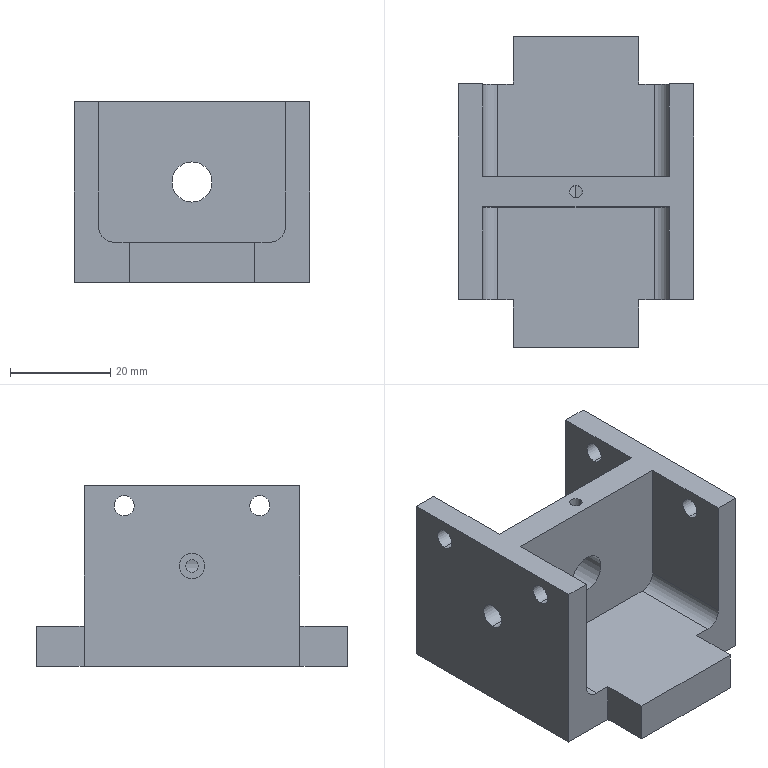Part | SolidWorks | features ICE 6, 3DProfileFeature 2, HoleWzd 2, Extrusion 1, Fillet 1 | 1 solid | 43 faces | box 47 x 62 x 36 mm | volume 37251 mm3 | plane 23 | cylinder 20 | commonest cylinder face diameters 4 x8 2.5 x4 6 x4 5 x2 8 x2
STEP:
#1=CARTESIAN_POINT('',(-9.5,0.,17.5));
#2=VERTEX_POINT('',#1);
#3=CARTESIAN_POINT('',(-9.5,0.,22.5));
#4=VERTEX_POINT('',#3);
#5=CARTESIAN_POINT('',(-9.5,0.,20.));
#6=DIRECTION('',(-1.,0.,0.));
#7=DIRECTION('',(0.,0.,1.));
#8=AXIS2_PLACEMENT_3D('',#5,#6,#7);
#9=CIRCLE('',#8,2.5);
#10=EDGE_CURVE('',#2,#4,#9,.T.);
#11=ORIENTED_EDGE('',*,*,#10,.F.);
#12=CARTESIAN_POINT('',(-23.5,0.,17.5));
#13=VERTEX_POINT('',#12);
#14=CARTESIAN_POINT('',(-9.5,0.,17.5));
#15=DIRECTION('',(-1.,0.,0.));
#16=VECTOR('',#15,1000.);
#17=LINE('',#14,#16);
#18=EDGE_CURVE('',#2,#13,#17,.T.);
#19=ORIENTED_EDGE('',*,*,#18,.T.);
#20=CARTESIAN_POINT('',(-23.5,0.,22.5));
#21=VERTEX_POINT('',#20);
#22=CARTESIAN_POINT('',(-23.5,0.,20.));
#23=DIRECTION('',(-1.,0.,0.));
#24=DIRECTION('',(0.,0.,1.));
#25=AXIS2_PLACEMENT_3D('',#22,#23,#24);
#26=CIRCLE('',#25,2.5);
#27=EDGE_CURVE('',#13,#21,#26,.T.);
#28=ORIENTED_EDGE('',*,*,#27,.T.);
#29=CARTESIAN_POINT('',(-9.5,0.,22.5));
#30=DIRECTION('',(-1.,0.,0.));
#31=VECTOR('',#30,1000.);
#32=LINE('',#29,#31);
#33=EDGE_CURVE('',#4,#21,#32,.T.);
#34=ORIENTED_EDGE('',*,*,#33,.F.);
#35=EDGE_LOOP('',(#11,#19,#28,#34));
#36=FACE_OUTER_BOUND('',#35,.T.);
#37=CARTESIAN_POINT('',(-9.5,0.,20.));
#38=DIRECTION('',(-1.,0.,0.));
#39=DIRECTION('',(0.,0.,1.));
#40=AXIS2_PLACEMENT_3D('',#37,#38,#39);
#41=CYLINDRICAL_SURFACE('',#40,2.5);
#42=ADVANCED_FACE('',(#36),#41,.F.);
#43=CARTESIAN_POINT('',(-1.25,0.,23.8));
#44=VERTEX_POINT('',#43);
#45=CARTESIAN_POINT('',(0.,-1.25,24.));
#46=VERTEX_POINT('',#45);
#47=CARTESIAN_POINT('',(-1.25,0.,23.8));
#48=CARTESIAN_POINT('',(-1.25,-0.1648,23.8));
#49=CARTESIAN_POINT('',(-1.217,-0.3295,23.811));
#50=CARTESIAN_POINT('',(-1.092,-0.6305,23.849));
#51=CARTESIAN_POINT('',(-0.9987,-0.769,23.875));
#52=CARTESIAN_POINT('',(-0.7696,-0.9982,23.927));
#53=CARTESIAN_POINT('',(-0.6317,-1.091,23.953));
#54=CARTESIAN_POINT('',(-0.3299,-1.217,23.989));
#55=CARTESIAN_POINT('',(-0.1663,-1.25,24.));
#56=CARTESIAN_POINT('',(0.,-1.25,24.));
#57=B_SPLINE_CURVE_WITH_KNOTS('',3,(#47,#48,#49,#50,#51,#52,#53,#54,#55,#56),.UNSPECIFIED.,.F.,.F.,(4,2,2,2,4),(0.005899,0.00639,0.006882,0.007373,0.007865),.UNSPECIFIED.);
#58=EDGE_CURVE('',#44,#46,#57,.T.);
#59=ORIENTED_EDGE('',*,*,#58,.F.);
#60=CARTESIAN_POINT('',(-1.25,0.,36.));
#61=VERTEX_POINT('',#60);
#62=CARTESIAN_POINT('',(-1.25,0.,36.));
#63=DIRECTION('',(0.,0.,1.));
#64=VECTOR('',#63,1000.);
#65=LINE('',#62,#64);
#66=EDGE_CURVE('',#44,#61,#65,.T.);
#67=ORIENTED_EDGE('',*,*,#66,.T.);
#68=CARTESIAN_POINT('',(1.25,0.,36.));
#69=VERTEX_POINT('',#68);
#70=CARTESIAN_POINT('',(0.,0.,36.));
#71=DIRECTION('',(0.,0.,1.));
#72=DIRECTION('',(1.,0.,0.));
#73=AXIS2_PLACEMENT_3D('',#70,#71,#72);
#74=CIRCLE('',#73,1.25);
#75=EDGE_CURVE('',#61,#69,#74,.T.);
#76=ORIENTED_EDGE('',*,*,#75,.T.);
#77=CARTESIAN_POINT('',(1.25,0.,23.8));
#78=VERTEX_POINT('',#77);
#79=CARTESIAN_POINT('',(1.25,0.,36.));
#80=DIRECTION('',(0.,0.,1.));
#81=VECTOR('',#80,1000.);
#82=LINE('',#79,#81);
#83=EDGE_CURVE('',#78,#69,#82,.T.);
#84=ORIENTED_EDGE('',*,*,#83,.F.);
#85=CARTESIAN_POINT('',(0.,-1.25,24.));
#86=CARTESIAN_POINT('',(0.1664,-1.25,24.));
#87=CARTESIAN_POINT('',(0.3295,-1.217,23.989));
#88=CARTESIAN_POINT('',(0.6319,-1.091,23.953));
#89=CARTESIAN_POINT('',(0.7699,-0.998,23.927));
#90=CARTESIAN_POINT('',(0.9989,-0.7687,23.875));
#91=CARTESIAN_POINT('',(1.092,-0.63,23.849));
#92=CARTESIAN_POINT('',(1.217,-0.3295,23.811));
#93=CARTESIAN_POINT('',(1.25,-0.1643,23.8));
#94=CARTESIAN_POINT('',(1.25,0.,23.8));
#95=B_SPLINE_CURVE_WITH_KNOTS('',3,(#85,#86,#87,#88,#89,#90,#91,#92,#93,#94),.UNSPECIFIED.,.F.,.F.,(4,2,2,2,4),(0.,0.0004918,0.0009835,0.001475,0.001967),.UNSPECIFIED.);
#96=EDGE_CURVE('',#46,#78,#95,.T.);
#97=ORIENTED_EDGE('',*,*,#96,.F.);
#98=EDGE_LOOP('',(#59,#67,#76,#84,#97));
#99=FACE_OUTER_BOUND('',#98,.T.);
#100=CARTESIAN_POINT('',(0.,0.,36.));
#101=DIRECTION('',(0.,0.,1.));
#102=DIRECTION('',(1.,0.,0.));
#103=AXIS2_PLACEMENT_3D('',#100,#101,#102);
#104=CYLINDRICAL_SURFACE('',#103,1.25);
#105=ADVANCED_FACE('',(#99),#104,.F.);
#106=CARTESIAN_POINT('',(-3.8,0.,21.25));
#107=VERTEX_POINT('',#106);
#108=CARTESIAN_POINT('',(-3.8,0.,18.75));
#109=VERTEX_POINT('',#108);
#110=CARTESIAN_POINT('',(-3.8,0.,21.25));
#111=CARTESIAN_POINT('',(-3.8,0.1663,21.25));
#112=CARTESIAN_POINT('',(-3.811,0.3294,21.217));
#113=CARTESIAN_POINT('',(-3.849,0.6316,21.091));
#114=CARTESIAN_POINT('',(-3.875,0.7696,20.998));
#115=CARTESIAN_POINT('',(-3.927,0.9986,20.769));
#116=CARTESIAN_POINT('',(-3.953,1.092,20.631));
#117=CARTESIAN_POINT('',(-3.989,1.217,20.33));
#118=CARTESIAN_POINT('',(-4.,1.25,20.165));
#119=CARTESIAN_POINT('',(-4.,1.25,19.918));
#120=CARTESIAN_POINT('',(-3.997,1.242,19.835));
#121=CARTESIAN_POINT('',(-3.988,1.21,19.674));
#122=CARTESIAN_POINT('',(-3.98,1.186,19.596));
#123=CARTESIAN_POINT('',(-3.953,1.091,19.368));
#124=CARTESIAN_POINT('',(-3.927,0.9987,19.231));
#125=CARTESIAN_POINT('',(-3.888,0.8257,19.058));
#126=CARTESIAN_POINT('',(-3.875,0.7631,19.007));
#127=CARTESIAN_POINT('',(-3.851,0.6281,18.916));
#128=CARTESIAN_POINT('',(-3.839,0.555,18.877));
#129=CARTESIAN_POINT('',(-3.811,0.3291,18.783));
#130=CARTESIAN_POINT('',(-3.8,0.1638,18.75));
#131=CARTESIAN_POINT('',(-3.8,0.,18.75));
#132=B_SPLINE_CURVE_WITH_KNOTS('',3,(#110,#111,#112,#113,#114,#115,#116,#117,#118,#119,#120,#121,#122,#123,#124,#125,#126,#127,#128,#129,#130,#131),.UNSPECIFIED.,.F.,.F.,(4,2,2,2,2,2,2,2,2,2,4),(0.,0.0004916,0.0009832,0.001475,0.001966,0.002212,0.002458,0.00295,0.003195,0.003441,0.003933),.UNSPECIFIED.);
#133=EDGE_CURVE('',#107,#109,#132,.T.);
#134=ORIENTED_EDGE('',*,*,#133,.T.);
#135=CARTESIAN_POINT('',(-3.8,0.,18.75));
#136=CARTESIAN_POINT('',(-3.8,-0.1638,18.75));
#137=CARTESIAN_POINT('',(-3.811,-0.3292,18.783));
#138=CARTESIAN_POINT('',(-3.849,-0.6305,18.908));
#139=CARTESIAN_POINT('',(-3.875,-0.7683,19.001));
#140=CARTESIAN_POINT('',(-3.927,-0.9991,19.231));
#141=CARTESIAN_POINT('',(-3.953,-1.091,19.368));
#142=CARTESIAN_POINT('',(-3.98,-1.186,19.596));
#143=CARTESIAN_POINT('',(-3.988,-1.21,19.674));
#144=CARTESIAN_POINT('',(-3.997,-1.242,19.834));
#145=CARTESIAN_POINT('',(-4.,-1.25,19.918));
#146=CARTESIAN_POINT('',(-4.,-1.25,20.165));
#147=CARTESIAN_POINT('',(-3.989,-1.217,20.33));
#148=CARTESIAN_POINT('',(-3.953,-1.091,20.631));
#149=CARTESIAN_POINT('',(-3.927,-0.9985,20.769));
#150=CARTESIAN_POINT('',(-3.875,-0.7694,20.998));
#151=CARTESIAN_POINT('',(-3.849,-0.6315,21.091));
#152=CARTESIAN_POINT('',(-3.811,-0.3299,21.217));
#153=CARTESIAN_POINT('',(-3.8,-0.1663,21.25));
#154=CARTESIAN_POINT('',(-3.8,0.,21.25));
#155=B_SPLINE_CURVE_WITH_KNOTS('',3,(#135,#136,#137,#138,#139,#140,#141,#142,#143,#144,#145,#146,#147,#148,#149,#150,#151,#152,#153,#154),.UNSPECIFIED.,.F.,.F.,(4,2,2,2,2,2,2,2,2,4),(0.003933,0.004424,0.004916,0.005407,0.005653,0.005899,0.00639,0.006882,0.007373,0.007864),.UNSPECIFIED.);
#156=EDGE_CURVE('',#109,#107,#155,.T.);
#157=ORIENTED_EDGE('',*,*,#156,.T.);
#158=EDGE_LOOP('',(#134,#157));
#159=FACE_BOUND('',#158,.T.);
#160=CARTESIAN_POINT('',(0.,-3.,24.));
#161=VERTEX_POINT('',#160);
#162=CARTESIAN_POINT('',(0.,-3.,16.));
#163=VERTEX_POINT('',#162);
#164=CARTESIAN_POINT('',(0.,-3.,20.));
#165=DIRECTION('',(0.,-1.,0.));
#166=DIRECTION('',(0.,0.,1.));
#167=AXIS2_PLACEMENT_3D('',#164,#165,#166);
#168=CIRCLE('',#167,4.);
#169=EDGE_CURVE('',#161,#163,#168,.T.);
#170=ORIENTED_EDGE('',*,*,#169,.T.);
#171=CARTESIAN_POINT('',(0.,3.,16.));
#172=VERTEX_POINT('',#171);
#173=CARTESIAN_POINT('',(0.,-21.501,16.));
#174=DIRECTION('',(0.,1.,0.));
#175=VECTOR('',#174,1000.);
#176=LINE('',#173,#175);
#177=EDGE_CURVE('',#163,#172,#176,.T.);
#178=ORIENTED_EDGE('',*,*,#177,.T.);
#179=CARTESIAN_POINT('',(0.,3.,24.));
#180=VERTEX_POINT('',#179);
#181=CARTESIAN_POINT('',(0.,3.,20.));
#182=DIRECTION('',(0.,1.,0.));
#183=DIRECTION('',(0.,0.,1.));
#184=AXIS2_PLACEMENT_3D('',#181,#182,#183);
#185=CIRCLE('',#184,4.);
#186=EDGE_CURVE('',#172,#180,#185,.T.);
#187=ORIENTED_EDGE('',*,*,#186,.T.);
#188=CARTESIAN_POINT('',(0.,1.25,24.));
#189=VERTEX_POINT('',#188);
#190=CARTESIAN_POINT('',(0.,-21.501,24.));
#191=DIRECTION('',(0.,1.,0.));
#192=VECTOR('',#191,1000.);
#193=LINE('',#190,#192);
#194=EDGE_CURVE('',#189,#180,#193,.T.);
#195=ORIENTED_EDGE('',*,*,#194,.F.);
#196=CARTESIAN_POINT('',(0.,1.25,24.));
#197=CARTESIAN_POINT('',(-0.1638,1.25,24.));
#198=CARTESIAN_POINT('',(-0.3292,1.217,23.989));
#199=CARTESIAN_POINT('',(-0.6307,1.092,23.953));
#200=CARTESIAN_POINT('',(-0.7685,0.9993,23.927));
#201=CARTESIAN_POINT('',(-0.9992,0.7685,23.875));
#202=CARTESIAN_POINT('',(-1.091,0.6322,23.849));
#203=CARTESIAN_POINT('',(-1.186,0.404,23.82));
#204=CARTESIAN_POINT('',(-1.21,0.3258,23.813));
#205=CARTESIAN_POINT('',(-1.242,0.1656,23.802));
#206=CARTESIAN_POINT('',(-1.25,0.08238,23.8));
#207=CARTESIAN_POINT('',(-1.25,0.,23.8));
#208=B_SPLINE_CURVE_WITH_KNOTS('',3,(#196,#197,#198,#199,#200,#201,#202,#203,#204,#205,#206,#207),.UNSPECIFIED.,.F.,.F.,(4,2,2,2,2,4),(0.003933,0.004424,0.004916,0.005407,0.005653,0.005899),.UNSPECIFIED.);
#209=EDGE_CURVE('',#189,#44,#208,.T.);
#210=ORIENTED_EDGE('',*,*,#209,.T.);
#211=ORIENTED_EDGE('',*,*,#58,.T.);
#212=CARTESIAN_POINT('',(0.,-21.501,24.));
#213=DIRECTION('',(0.,1.,0.));
#214=VECTOR('',#213,1000.);
#215=LINE('',#212,#214);
#216=EDGE_CURVE('',#161,#46,#215,.T.);
#217=ORIENTED_EDGE('',*,*,#216,.F.);
#218=EDGE_LOOP('',(#170,#178,#187,#195,#210,#211,#217));
#219=FACE_OUTER_BOUND('',#218,.T.);
#220=CARTESIAN_POINT('',(0.,-21.501,20.));
#221=DIRECTION('',(0.,1.,0.));
#222=DIRECTION('',(0.,0.,1.));
#223=AXIS2_PLACEMENT_3D('',#220,#221,#222);
#224=CYLINDRICAL_SURFACE('',#223,4.);
#225=ADVANCED_FACE('',(#159,#219),#224,.F.);
#226=CARTESIAN_POINT('',(23.5,13.5,34.));
#227=VERTEX_POINT('',#226);
#228=CARTESIAN_POINT('',(23.5,13.5,30.));
#229=VERTEX_POINT('',#228);
#230=CARTESIAN_POINT('',(23.5,13.5,32.));
#231=DIRECTION('',(1.,0.,0.));
#232=DIRECTION('',(0.,0.,1.));
#233=AXIS2_PLACEMENT_3D('',#230,#231,#232);
#234=CIRCLE('',#233,2.);
#235=EDGE_CURVE('',#227,#229,#234,.T.);
#236=ORIENTED_EDGE('',*,*,#235,.T.);
#237=CARTESIAN_POINT('',(18.6,13.5,30.));
#238=VERTEX_POINT('',#237);
#239=CARTESIAN_POINT('',(29.157,13.5,30.));
#240=DIRECTION('',(-1.,0.,0.));
#241=VECTOR('',#240,1000.);
#242=LINE('',#239,#241);
#243=EDGE_CURVE('',#229,#238,#242,.T.);
#244=ORIENTED_EDGE('',*,*,#243,.T.);
#245=CARTESIAN_POINT('',(18.6,13.5,34.));
#246=VERTEX_POINT('',#245);
#247=CARTESIAN_POINT('',(18.6,13.5,32.));
#248=DIRECTION('',(1.,0.,0.));
#249=DIRECTION('',(0.,0.,-1.));
#250=AXIS2_PLACEMENT_3D('',#247,#248,#249);
#251=CIRCLE('',#250,2.);
#252=EDGE_CURVE('',#246,#238,#251,.T.);
#253=ORIENTED_EDGE('',*,*,#252,.F.);
#254=CARTESIAN_POINT('',(29.157,13.5,34.));
#255=DIRECTION('',(-1.,0.,0.));
#256=VECTOR('',#255,1000.);
#257=LINE('',#254,#256);
#258=EDGE_CURVE('',#227,#246,#257,.T.);
#259=ORIENTED_EDGE('',*,*,#258,.F.);
#260=EDGE_LOOP('',(#236,#244,#253,#259));
#261=FACE_OUTER_BOUND('',#260,.T.);
#262=CARTESIAN_POINT('',(29.157,13.5,32.));
#263=DIRECTION('',(-1.,0.,0.));
#264=DIRECTION('',(0.,0.,1.));
#265=AXIS2_PLACEMENT_3D('',#262,#263,#264);
#266=CYLINDRICAL_SURFACE('',#265,2.);
#267=ADVANCED_FACE('',(#261),#266,.F.);
#268=CARTESIAN_POINT('',(23.5,-13.5,34.));
#269=VERTEX_POINT('',#268);
#270=CARTESIAN_POINT('',(23.5,-13.5,30.));
#271=VERTEX_POINT('',#270);
#272=CARTESIAN_POINT('',(23.5,-13.5,32.));
#273=DIRECTION('',(1.,0.,0.));
#274=DIRECTION('',(0.,0.,1.));
#275=AXIS2_PLACEMENT_3D('',#272,#273,#274);
#276=CIRCLE('',#275,2.);
#277=EDGE_CURVE('',#269,#271,#276,.T.);
#278=ORIENTED_EDGE('',*,*,#277,.T.);
#279=CARTESIAN_POINT('',(18.6,-13.5,30.));
#280=VERTEX_POINT('',#279);
#281=CARTESIAN_POINT('',(29.157,-13.5,30.));
#282=DIRECTION('',(-1.,0.,0.));
#283=VECTOR('',#282,1000.);
#284=LINE('',#281,#283);
#285=EDGE_CURVE('',#271,#280,#284,.T.);
#286=ORIENTED_EDGE('',*,*,#285,.T.);
#287=CARTESIAN_POINT('',(18.6,-13.5,34.));
#288=VERTEX_POINT('',#287);
#289=CARTESIAN_POINT('',(18.6,-13.5,32.));
#290=DIRECTION('',(1.,0.,0.));
#291=DIRECTION('',(0.,0.,-1.));
#292=AXIS2_PLACEMENT_3D('',#289,#290,#291);
#293=CIRCLE('',#292,2.);
#294=EDGE_CURVE('',#288,#280,#293,.T.);
#295=ORIENTED_EDGE('',*,*,#294,.F.);
#296=CARTESIAN_POINT('',(29.157,-13.5,34.));
#297=DIRECTION('',(-1.,0.,0.));
#298=VECTOR('',#297,1000.);
#299=LINE('',#296,#298);
#300=EDGE_CURVE('',#269,#288,#299,.T.);
#301=ORIENTED_EDGE('',*,*,#300,.F.);
#302=EDGE_LOOP('',(#278,#286,#295,#301));
#303=FACE_OUTER_BOUND('',#302,.T.);
#304=CARTESIAN_POINT('',(29.157,-13.5,32.));
#305=DIRECTION('',(-1.,0.,0.));
#306=DIRECTION('',(0.,0.,1.));
#307=AXIS2_PLACEMENT_3D('',#304,#305,#306);
#308=CYLINDRICAL_SURFACE('',#307,2.);
#309=ADVANCED_FACE('',(#303),#308,.F.);
#310=CARTESIAN_POINT('',(-18.6,13.5,30.));
#311=VERTEX_POINT('',#310);
#312=CARTESIAN_POINT('',(-18.6,13.5,34.));
#313=VERTEX_POINT('',#312);
#314=CARTESIAN_POINT('',(-18.6,13.5,32.));
#315=DIRECTION('',(-1.,0.,0.));
#316=DIRECTION('',(0.,0.,1.));
#317=AXIS2_PLACEMENT_3D('',#314,#315,#316);
#318=CIRCLE('',#317,2.);
#319=EDGE_CURVE('',#311,#313,#318,.T.);
#320=ORIENTED_EDGE('',*,*,#319,.F.);
#321=CARTESIAN_POINT('',(-23.5,13.5,30.));
#322=VERTEX_POINT('',#321);
#323=CARTESIAN_POINT('',(29.157,13.5,30.));
#324=DIRECTION('',(-1.,0.,0.));
#325=VECTOR('',#324,1000.);
#326=LINE('',#323,#325);
#327=EDGE_CURVE('',#311,#322,#326,.T.);
#328=ORIENTED_EDGE('',*,*,#327,.T.);
#329=CARTESIAN_POINT('',(-23.5,13.5,34.));
#330=VERTEX_POINT('',#329);
#331=CARTESIAN_POINT('',(-23.5,13.5,32.));
#332=DIRECTION('',(-1.,0.,0.));
#333=DIRECTION('',(0.,0.,1.));
#334=AXIS2_PLACEMENT_3D('',#331,#332,#333);
#335=CIRCLE('',#334,2.);
#336=EDGE_CURVE('',#322,#330,#335,.T.);
#337=ORIENTED_EDGE('',*,*,#336,.T.);
#338=CARTESIAN_POINT('',(29.157,13.5,34.));
#339=DIRECTION('',(-1.,0.,0.));
#340=VECTOR('',#339,1000.);
#341=LINE('',#338,#340);
#342=EDGE_CURVE('',#313,#330,#341,.T.);
#343=ORIENTED_EDGE('',*,*,#342,.F.);
#344=EDGE_LOOP('',(#320,#328,#337,#343));
#345=FACE_OUTER_BOUND('',#344,.T.);
#346=CARTESIAN_POINT('',(29.157,13.5,32.));
#347=DIRECTION('',(-1.,0.,0.));
#348=DIRECTION('',(0.,0.,1.));
#349=AXIS2_PLACEMENT_3D('',#346,#347,#348);
#350=CYLINDRICAL_SURFACE('',#349,2.);
#351=ADVANCED_FACE('',(#345),#350,.F.);
#352=CARTESIAN_POINT('',(-18.6,-13.5,30.));
#353=VERTEX_POINT('',#352);
#354=CARTESIAN_POINT('',(-18.6,-13.5,34.));
#355=VERTEX_POINT('',#354);
#356=CARTESIAN_POINT('',(-18.6,-13.5,32.));
#357=DIRECTION('',(-1.,0.,0.));
#358=DIRECTION('',(0.,0.,1.));
#359=AXIS2_PLACEMENT_3D('',#356,#357,#358);
#360=CIRCLE('',#359,2.);
#361=EDGE_CURVE('',#353,#355,#360,.T.);
#362=ORIENTED_EDGE('',*,*,#361,.F.);
#363=CARTESIAN_POINT('',(-23.5,-13.5,30.));
#364=VERTEX_POINT('',#363);
#365=CARTESIAN_POINT('',(29.157,-13.5,30.));
#366=DIRECTION('',(-1.,0.,0.));
#367=VECTOR('',#366,1000.);
#368=LINE('',#365,#367);
#369=EDGE_CURVE('',#353,#364,#368,.T.);
#370=ORIENTED_EDGE('',*,*,#369,.T.);
#371=CARTESIAN_POINT('',(-23.5,-13.5,34.));
#372=VERTEX_POINT('',#371);
#373=CARTESIAN_POINT('',(-23.5,-13.5,32.));
#374=DIRECTION('',(-1.,0.,0.));
#375=DIRECTION('',(0.,0.,-1.));
#376=AXIS2_PLACEMENT_3D('',#373,#374,#375);
#377=CIRCLE('',#376,2.);
#378=EDGE_CURVE('',#364,#372,#377,.T.);
#379=ORIENTED_EDGE('',*,*,#378,.T.);
#380=CARTESIAN_POINT('',(29.157,-13.5,34.));
#381=DIRECTION('',(-1.,0.,0.));
#382=VECTOR('',#381,1000.);
#383=LINE('',#380,#382);
#384=EDGE_CURVE('',#355,#372,#383,.T.);
#385=ORIENTED_EDGE('',*,*,#384,.F.);
#386=EDGE_LOOP('',(#362,#370,#379,#385));
#387=FACE_OUTER_BOUND('',#386,.T.);
#388=CARTESIAN_POINT('',(29.157,-13.5,32.));
#389=DIRECTION('',(-1.,0.,0.));
#390=DIRECTION('',(0.,0.,1.));
#391=AXIS2_PLACEMENT_3D('',#388,#389,#390);
#392=CYLINDRICAL_SURFACE('',#391,2.);
#393=ADVANCED_FACE('',(#387),#392,.F.);
#394=ORIENTED_EDGE('',*,*,#156,.F.);
#395=CARTESIAN_POINT('',(-9.5,0.,18.75));
#396=VERTEX_POINT('',#395);
#397=CARTESIAN_POINT('',(-23.5,0.,18.75));
#398=DIRECTION('',(-1.,0.,0.));
#399=VECTOR('',#398,1000.);
#400=LINE('',#397,#399);
#401=EDGE_CURVE('',#109,#396,#400,.T.);
#402=ORIENTED_EDGE('',*,*,#401,.T.);
#403=CARTESIAN_POINT('',(-9.5,0.,21.25));
#404=VERTEX_POINT('',#403);
#405=CARTESIAN_POINT('',(-9.5,0.,20.));
#406=DIRECTION('',(1.,0.,0.));
#407=DIRECTION('',(0.,0.,1.));
#408=AXIS2_PLACEMENT_3D('',#405,#406,#407);
#409=CIRCLE('',#408,1.25);
#410=EDGE_CURVE('',#404,#396,#409,.T.);
#411=ORIENTED_EDGE('',*,*,#410,.F.);
#412=CARTESIAN_POINT('',(-23.5,0.,21.25));
#413=DIRECTION('',(-1.,0.,0.));
#414=VECTOR('',#413,1000.);
#415=LINE('',#412,#414);
#416=EDGE_CURVE('',#107,#404,#415,.T.);
#417=ORIENTED_EDGE('',*,*,#416,.F.);
#418=EDGE_LOOP('',(#394,#402,#411,#417));
#419=FACE_OUTER_BOUND('',#418,.T.);
#420=CARTESIAN_POINT('',(-23.5,0.,20.));
#421=DIRECTION('',(-1.,0.,0.));
#422=DIRECTION('',(0.,0.,1.));
#423=AXIS2_PLACEMENT_3D('',#420,#421,#422);
#424=CYLINDRICAL_SURFACE('',#423,1.25);
#425=ADVANCED_FACE('',(#419),#424,.F.);
#426=ORIENTED_EDGE('',*,*,#401,.F.);
#427=ORIENTED_EDGE('',*,*,#133,.F.);
#428=ORIENTED_EDGE('',*,*,#416,.T.);
#429=CARTESIAN_POINT('',(-9.5,0.,20.));
#430=DIRECTION('',(1.,0.,0.));
#431=DIRECTION('',(0.,0.,1.));
#432=AXIS2_PLACEMENT_3D('',#429,#430,#431);
#433=CIRCLE('',#432,1.25);
#434=EDGE_CURVE('',#396,#404,#433,.T.);
#435=ORIENTED_EDGE('',*,*,#434,.F.);
#436=EDGE_LOOP('',(#426,#427,#428,#435));
#437=FACE_OUTER_BOUND('',#436,.T.);
#438=CARTESIAN_POINT('',(-23.5,0.,20.));
#439=DIRECTION('',(-1.,0.,0.));
#440=DIRECTION('',(0.,0.,1.));
#441=AXIS2_PLACEMENT_3D('',#438,#439,#440);
#442=CYLINDRICAL_SURFACE('',#441,1.25);
#443=ADVANCED_FACE('',(#437),#442,.F.);
#444=CARTESIAN_POINT('',(-12.5,-21.5,8.));
#445=VERTEX_POINT('',#444);
#446=CARTESIAN_POINT('',(-12.5,-21.5,0.));
#447=VERTEX_POINT('',#446);
#448=CARTESIAN_POINT('',(-12.5,-21.5,34.744));
#449=DIRECTION('',(0.,0.,-1.));
#450=VECTOR('',#449,1000.);
#451=LINE('',#448,#450);
#452=EDGE_CURVE('',#445,#447,#451,.T.);
#453=ORIENTED_EDGE('',*,*,#452,.F.);
#454=CARTESIAN_POINT('',(-15.6,-21.5,8.));
#455=VERTEX_POINT('',#454);
#456=CARTESIAN_POINT('',(-18.6,-21.5,8.));
#457=DIRECTION('',(1.,0.,0.));
#458=VECTOR('',#457,1000.);
#459=LINE('',#456,#458);
#460=EDGE_CURVE('',#455,#445,#459,.T.);
#461=ORIENTED_EDGE('',*,*,#460,.F.);
#462=CARTESIAN_POINT('',(-18.6,-21.5,11.));
#463=VERTEX_POINT('',#462);
#464=CARTESIAN_POINT('',(-15.6,-21.5,11.));
#465=DIRECTION('',(0.,1.,0.));
#466=DIRECTION('',(0.,0.,1.));
#467=AXIS2_PLACEMENT_3D('',#464,#465,#466);
#468=CIRCLE('',#467,3.);
#469=EDGE_CURVE('',#455,#463,#468,.T.);
#470=ORIENTED_EDGE('',*,*,#469,.T.);
#471=CARTESIAN_POINT('',(-18.6,-21.5,36.));
#472=VERTEX_POINT('',#471);
#473=CARTESIAN_POINT('',(-18.6,-21.5,8.));
#474=DIRECTION('',(0.,0.,1.));
#475=VECTOR('',#474,1000.);
#476=LINE('',#473,#475);
#477=EDGE_CURVE('',#463,#472,#476,.T.);
#478=ORIENTED_EDGE('',*,*,#477,.T.);
#479=CARTESIAN_POINT('',(-23.5,-21.5,36.));
#480=VERTEX_POINT('',#479);
#481=CARTESIAN_POINT('',(-23.5,-21.5,36.));
#482=DIRECTION('',(1.,0.,0.));
#483=VECTOR('',#482,1000.);
#484=LINE('',#481,#483);
#485=EDGE_CURVE('',#480,#472,#484,.T.);
#486=ORIENTED_EDGE('',*,*,#485,.F.);
#487=CARTESIAN_POINT('',(-23.5,-21.5,0.));
#488=VERTEX_POINT('',#487);
#489=CARTESIAN_POINT('',(-23.5,-21.5,36.));
#490=DIRECTION('',(0.,0.,-1.));
#491=VECTOR('',#490,1000.);
#492=LINE('',#489,#491);
#493=EDGE_CURVE('',#480,#488,#492,.T.);
#494=ORIENTED_EDGE('',*,*,#493,.T.);
#495=CARTESIAN_POINT('',(-23.5,-21.5,0.));
#496=DIRECTION('',(1.,0.,0.));
#497=VECTOR('',#496,1000.);
#498=LINE('',#495,#497);
#499=EDGE_CURVE('',#488,#447,#498,.T.);
#500=ORIENTED_EDGE('',*,*,#499,.T.);
#501=EDGE_LOOP('',(#453,#461,#470,#478,#486,#494,#500));
#502=FACE_OUTER_BOUND('',#501,.T.);
#503=CARTESIAN_POINT('',(-23.5,-21.5,36.));
#504=DIRECTION('',(0.,1.,0.));
#505=DIRECTION('',(0.,0.,1.));
#506=AXIS2_PLACEMENT_3D('',#503,#504,#505);
#507=PLANE('',#506);
#508=ADVANCED_FACE('',(#502),#507,.F.);
#509=CARTESIAN_POINT('',(12.5,21.5,8.));
#510=VERTEX_POINT('',#509);
#511=CARTESIAN_POINT('',(12.5,21.5,0.));
#512=VERTEX_POINT('',#511);
#513=CARTESIAN_POINT('',(12.5,21.5,34.744));
#514=DIRECTION('',(0.,0.,-1.));
#515=VECTOR('',#514,1000.);
#516=LINE('',#513,#515);
#517=EDGE_CURVE('',#510,#512,#516,.T.);
#518=ORIENTED_EDGE('',*,*,#517,.F.);
#519=CARTESIAN_POINT('',(15.6,21.5,8.));
#520=VERTEX_POINT('',#519);
#521=CARTESIAN_POINT('',(-18.6,21.5,8.));
#522=DIRECTION('',(-1.,0.,0.));
#523=VECTOR('',#522,1000.);
#524=LINE('',#521,#523);
#525=EDGE_CURVE('',#520,#510,#524,.T.);
#526=ORIENTED_EDGE('',*,*,#525,.F.);
#527=CARTESIAN_POINT('',(18.6,21.5,11.));
#528=VERTEX_POINT('',#527);
#529=CARTESIAN_POINT('',(15.6,21.5,11.));
#530=DIRECTION('',(0.,-1.,0.));
#531=DIRECTION('',(0.,0.,-1.));
#532=AXIS2_PLACEMENT_3D('',#529,#530,#531);
#533=CIRCLE('',#532,3.);
#534=EDGE_CURVE('',#520,#528,#533,.T.);
#535=ORIENTED_EDGE('',*,*,#534,.T.);
#536=CARTESIAN_POINT('',(18.6,21.5,36.));
#537=VERTEX_POINT('',#536);
#538=CARTESIAN_POINT('',(18.6,21.5,8.));
#539=DIRECTION('',(0.,0.,1.));
#540=VECTOR('',#539,1000.);
#541=LINE('',#538,#540);
#542=EDGE_CURVE('',#528,#537,#541,.T.);
#543=ORIENTED_EDGE('',*,*,#542,.T.);
#544=CARTESIAN_POINT('',(23.5,21.5,36.));
#545=VERTEX_POINT('',#544);
#546=CARTESIAN_POINT('',(-23.5,21.5,36.));
#547=DIRECTION('',(-1.,0.,0.));
#548=VECTOR('',#547,1000.);
#549=LINE('',#546,#548);
#550=EDGE_CURVE('',#545,#537,#549,.T.);
#551=ORIENTED_EDGE('',*,*,#550,.F.);
#552=CARTESIAN_POINT('',(23.5,21.5,0.));
#553=VERTEX_POINT('',#552);
#554=CARTESIAN_POINT('',(23.5,21.5,36.));
#555=DIRECTION('',(0.,0.,-1.));
#556=VECTOR('',#555,1000.);
#557=LINE('',#554,#556);
#558=EDGE_CURVE('',#545,#553,#557,.T.);
#559=ORIENTED_EDGE('',*,*,#558,.T.);
#560=CARTESIAN_POINT('',(-23.5,21.5,0.));
#561=DIRECTION('',(-1.,0.,0.));
#562=VECTOR('',#561,1000.);
#563=LINE('',#560,#562);
#564=EDGE_CURVE('',#553,#512,#563,.T.);
#565=ORIENTED_EDGE('',*,*,#564,.T.);
#566=EDGE_LOOP('',(#518,#526,#535,#543,#551,#559,#565));
#567=FACE_OUTER_BOUND('',#566,.T.);
#568=CARTESIAN_POINT('',(-23.5,21.5,36.));
#569=DIRECTION('',(0.,-1.,0.));
#570=DIRECTION('',(0.,0.,-1.));
#571=AXIS2_PLACEMENT_3D('',#568,#569,#570);
#572=PLANE('',#571);
#573=ADVANCED_FACE('',(#567),#572,.F.);
#574=ORIENTED_EDGE('',*,*,#485,.T.);
#575=CARTESIAN_POINT('',(-18.6,-3.,36.));
#576=VERTEX_POINT('',#575);
#577=CARTESIAN_POINT('',(-18.6,-21.5,36.));
#578=DIRECTION('',(0.,-1.,0.));
#579=VECTOR('',#578,1000.);
#580=LINE('',#577,#579);
#581=EDGE_CURVE('',#576,#472,#580,.T.);
#582=ORIENTED_EDGE('',*,*,#581,.F.);
#583=CARTESIAN_POINT('',(18.6,-3.,36.));
#584=VERTEX_POINT('',#583);
#585=CARTESIAN_POINT('',(-18.6,-3.,36.));
#586=DIRECTION('',(-1.,0.,0.));
#587=VECTOR('',#586,1000.);
#588=LINE('',#585,#587);
#589=EDGE_CURVE('',#584,#576,#588,.T.);
#590=ORIENTED_EDGE('',*,*,#589,.F.);
#591=CARTESIAN_POINT('',(18.6,-21.5,36.));
#592=VERTEX_POINT('',#591);
#593=CARTESIAN_POINT('',(18.6,-21.5,36.));
#594=DIRECTION('',(0.,1.,0.));
#595=VECTOR('',#594,1000.);
#596=LINE('',#593,#595);
#597=EDGE_CURVE('',#592,#584,#596,.T.);
#598=ORIENTED_EDGE('',*,*,#597,.F.);
#599=CARTESIAN_POINT('',(23.5,-21.5,36.));
#600=VERTEX_POINT('',#599);
#601=CARTESIAN_POINT('',(-23.5,-21.5,36.));
#602=DIRECTION('',(1.,0.,0.));
#603=VECTOR('',#602,1000.);
#604=LINE('',#601,#603);
#605=EDGE_CURVE('',#592,#600,#604,.T.);
#606=ORIENTED_EDGE('',*,*,#605,.T.);
#607=CARTESIAN_POINT('',(23.5,-21.5,36.));
#608=DIRECTION('',(0.,1.,0.));
#609=VECTOR('',#608,1000.);
#610=LINE('',#607,#609);
#611=EDGE_CURVE('',#600,#545,#610,.T.);
#612=ORIENTED_EDGE('',*,*,#611,.T.);
#613=ORIENTED_EDGE('',*,*,#550,.T.);
#614=CARTESIAN_POINT('',(18.6,3.,36.));
#615=VERTEX_POINT('',#614);
#616=CARTESIAN_POINT('',(18.6,-21.5,36.));
#617=DIRECTION('',(0.,1.,0.));
#618=VECTOR('',#617,1000.);
#619=LINE('',#616,#618);
#620=EDGE_CURVE('',#615,#537,#619,.T.);
#621=ORIENTED_EDGE('',*,*,#620,.F.);
#622=CARTESIAN_POINT('',(-18.6,3.,36.));
#623=VERTEX_POINT('',#622);
#624=CARTESIAN_POINT('',(-18.6,3.,36.));
#625=DIRECTION('',(1.,0.,0.));
#626=VECTOR('',#625,1000.);
#627=LINE('',#624,#626);
#628=EDGE_CURVE('',#623,#615,#627,.T.);
#629=ORIENTED_EDGE('',*,*,#628,.F.);
#630=CARTESIAN_POINT('',(-18.6,21.5,36.));
#631=VERTEX_POINT('',#630);
#632=CARTESIAN_POINT('',(-18.6,-21.5,36.));
#633=DIRECTION('',(0.,-1.,0.));
#634=VECTOR('',#633,1000.);
#635=LINE('',#632,#634);
#636=EDGE_CURVE('',#631,#623,#635,.T.);
#637=ORIENTED_EDGE('',*,*,#636,.F.);
#638=CARTESIAN_POINT('',(-23.5,21.5,36.));
#639=VERTEX_POINT('',#638);
#640=CARTESIAN_POINT('',(-23.5,21.5,36.));
#641=DIRECTION('',(-1.,0.,0.));
#642=VECTOR('',#641,1000.);
#643=LINE('',#640,#642);
#644=EDGE_CURVE('',#631,#639,#643,.T.);
#645=ORIENTED_EDGE('',*,*,#644,.T.);
#646=CARTESIAN_POINT('',(-23.5,-21.5,36.));
#647=DIRECTION('',(0.,-1.,0.));
#648=VECTOR('',#647,1000.);
#649=LINE('',#646,#648);
#650=EDGE_CURVE('',#639,#480,#649,.T.);
#651=ORIENTED_EDGE('',*,*,#650,.T.);
#652=EDGE_LOOP('',(#574,#582,#590,#598,#606,#612,#613,#621,#629,#637,#645,#651));
#653=FACE_OUTER_BOUND('',#652,.T.);
#654=CARTESIAN_POINT('',(0.,0.,36.));
#655=DIRECTION('',(0.,0.,1.));
#656=DIRECTION('',(1.,0.,0.));
#657=AXIS2_PLACEMENT_3D('',#654,#655,#656);
#658=CIRCLE('',#657,1.25);
#659=EDGE_CURVE('',#69,#61,#658,.T.);
#660=ORIENTED_EDGE('',*,*,#659,.F.);
#661=ORIENTED_EDGE('',*,*,#75,.F.);
#662=EDGE_LOOP('',(#660,#661));
#663=FACE_BOUND('',#662,.T.);
#664=CARTESIAN_POINT('',(0.,0.,36.));
#665=DIRECTION('',(0.,0.,-1.));
#666=DIRECTION('',(-1.,0.,0.));
#667=AXIS2_PLACEMENT_3D('',#664,#665,#666);
#668=PLANE('',#667);
#669=ADVANCED_FACE('',(#653,#663),#668,.F.);
#670=ORIENTED_EDGE('',*,*,#294,.T.);
#671=CARTESIAN_POINT('',(18.6,-13.5,32.));
#672=DIRECTION('',(1.,0.,0.));
#673=DIRECTION('',(0.,0.,-1.));
#674=AXIS2_PLACEMENT_3D('',#671,#672,#673);
#675=CIRCLE('',#674,2.);
#676=EDGE_CURVE('',#280,#288,#675,.T.);
#677=ORIENTED_EDGE('',*,*,#676,.T.);
#678=EDGE_LOOP('',(#670,#677));
#679=FACE_BOUND('',#678,.T.);
#680=CARTESIAN_POINT('',(18.6,-3.,11.));
#681=VERTEX_POINT('',#680);
#682=CARTESIAN_POINT('',(18.6,-3.,73.681));
#683=DIRECTION('',(0.,0.,-1.));
#684=VECTOR('',#683,1000.);
#685=LINE('',#682,#684);
#686=EDGE_CURVE('',#584,#681,#685,.T.);
#687=ORIENTED_EDGE('',*,*,#686,.T.);
#688=CARTESIAN_POINT('',(18.6,-21.5,11.));
#689=VERTEX_POINT('',#688);
#690=CARTESIAN_POINT('',(18.6,-21.5,11.));
#691=DIRECTION('',(0.,-1.,0.));
#692=VECTOR('',#691,1000.);
#693=LINE('',#690,#692);
#694=EDGE_CURVE('',#681,#689,#693,.T.);
#695=ORIENTED_EDGE('',*,*,#694,.T.);
#696=CARTESIAN_POINT('',(18.6,-21.5,8.));
#697=DIRECTION('',(0.,0.,1.));
#698=VECTOR('',#697,1000.);
#699=LINE('',#696,#698);
#700=EDGE_CURVE('',#689,#592,#699,.T.);
#701=ORIENTED_EDGE('',*,*,#700,.T.);
#702=ORIENTED_EDGE('',*,*,#597,.T.);
#703=EDGE_LOOP('',(#687,#695,#701,#702));
#704=FACE_OUTER_BOUND('',#703,.T.);
#705=CARTESIAN_POINT('',(18.6,-21.5,8.));
#706=DIRECTION('',(1.,0.,0.));
#707=DIRECTION('',(0.,0.,-1.));
#708=AXIS2_PLACEMENT_3D('',#705,#706,#707);
#709=PLANE('',#708);
#710=ADVANCED_FACE('',(#679,#704),#709,.F.);
#711=ORIENTED_EDGE('',*,*,#252,.T.);
#712=CARTESIAN_POINT('',(18.6,13.5,32.));
#713=DIRECTION('',(1.,0.,0.));
#714=DIRECTION('',(0.,0.,-1.));
#715=AXIS2_PLACEMENT_3D('',#712,#713,#714);
#716=CIRCLE('',#715,2.);
#717=EDGE_CURVE('',#238,#246,#716,.T.);
#718=ORIENTED_EDGE('',*,*,#717,.T.);
#719=EDGE_LOOP('',(#711,#718));
#720=FACE_BOUND('',#719,.T.);
#721=ORIENTED_EDGE('',*,*,#542,.F.);
#722=CARTESIAN_POINT('',(18.6,3.,11.));
#723=VERTEX_POINT('',#722);
#724=CARTESIAN_POINT('',(18.6,3.,11.));
#725=DIRECTION('',(0.,-1.,0.));
#726=VECTOR('',#725,1000.);
#727=LINE('',#724,#726);
#728=EDGE_CURVE('',#528,#723,#727,.T.);
#729=ORIENTED_EDGE('',*,*,#728,.T.);
#730=CARTESIAN_POINT('',(18.6,3.,73.681));
#731=DIRECTION('',(0.,0.,-1.));
#732=VECTOR('',#731,1000.);
#733=LINE('',#730,#732);
#734=EDGE_CURVE('',#615,#723,#733,.T.);
#735=ORIENTED_EDGE('',*,*,#734,.F.);
#736=ORIENTED_EDGE('',*,*,#620,.T.);
#737=EDGE_LOOP('',(#721,#729,#735,#736));
#738=FACE_OUTER_BOUND('',#737,.T.);
#739=CARTESIAN_POINT('',(18.6,-21.5,8.));
#740=DIRECTION('',(1.,0.,0.));
#741=DIRECTION('',(0.,0.,-1.));
#742=AXIS2_PLACEMENT_3D('',#739,#740,#741);
#743=PLANE('',#742);
#744=ADVANCED_FACE('',(#720,#738),#743,.F.);
#745=CARTESIAN_POINT('',(-18.6,-13.5,32.));
#746=DIRECTION('',(-1.,0.,0.));
#747=DIRECTION('',(0.,0.,1.));
#748=AXIS2_PLACEMENT_3D('',#745,#746,#747);
#749=CIRCLE('',#748,2.);
#750=EDGE_CURVE('',#355,#353,#749,.T.);
#751=ORIENTED_EDGE('',*,*,#750,.T.);
#752=ORIENTED_EDGE('',*,*,#361,.T.);
#753=EDGE_LOOP('',(#751,#752));
#754=FACE_BOUND('',#753,.T.);
#755=ORIENTED_EDGE('',*,*,#477,.F.);
#756=CARTESIAN_POINT('',(-18.6,-3.,11.));
#757=VERTEX_POINT('',#756);
#758=CARTESIAN_POINT('',(-18.6,-3.,11.));
#759=DIRECTION('',(0.,1.,0.));
#760=VECTOR('',#759,1000.);
#761=LINE('',#758,#760);
#762=EDGE_CURVE('',#463,#757,#761,.T.);
#763=ORIENTED_EDGE('',*,*,#762,.T.);
#764=CARTESIAN_POINT('',(-18.6,-3.,73.681));
#765=DIRECTION('',(0.,0.,-1.));
#766=VECTOR('',#765,1000.);
#767=LINE('',#764,#766);
#768=EDGE_CURVE('',#576,#757,#767,.T.);
#769=ORIENTED_EDGE('',*,*,#768,.F.);
#770=ORIENTED_EDGE('',*,*,#581,.T.);
#771=EDGE_LOOP('',(#755,#763,#769,#770));
#772=FACE_OUTER_BOUND('',#771,.T.);
#773=CARTESIAN_POINT('',(-18.6,-21.5,8.));
#774=DIRECTION('',(-1.,0.,0.));
#775=DIRECTION('',(0.,0.,1.));
#776=AXIS2_PLACEMENT_3D('',#773,#774,#775);
#777=PLANE('',#776);
#778=ADVANCED_FACE('',(#754,#772),#777,.F.);
#779=CARTESIAN_POINT('',(-18.6,13.5,32.));
#780=DIRECTION('',(-1.,0.,0.));
#781=DIRECTION('',(0.,0.,1.));
#782=AXIS2_PLACEMENT_3D('',#779,#780,#781);
#783=CIRCLE('',#782,2.);
#784=EDGE_CURVE('',#313,#311,#783,.T.);
#785=ORIENTED_EDGE('',*,*,#784,.T.);
#786=ORIENTED_EDGE('',*,*,#319,.T.);
#787=EDGE_LOOP('',(#785,#786));
#788=FACE_BOUND('',#787,.T.);
#789=CARTESIAN_POINT('',(-18.6,3.,11.));
#790=VERTEX_POINT('',#789);
#791=CARTESIAN_POINT('',(-18.6,3.,73.681));
#792=DIRECTION('',(0.,0.,-1.));
#793=VECTOR('',#792,1000.);
#794=LINE('',#791,#793);
#795=EDGE_CURVE('',#623,#790,#794,.T.);
#796=ORIENTED_EDGE('',*,*,#795,.T.);
#797=CARTESIAN_POINT('',(-18.6,21.5,11.));
#798=VERTEX_POINT('',#797);
#799=CARTESIAN_POINT('',(-18.6,21.5,11.));
#800=DIRECTION('',(0.,1.,0.));
#801=VECTOR('',#800,1000.);
#802=LINE('',#799,#801);
#803=EDGE_CURVE('',#790,#798,#802,.T.);
#804=ORIENTED_EDGE('',*,*,#803,.T.);
#805=CARTESIAN_POINT('',(-18.6,21.5,8.));
#806=DIRECTION('',(0.,0.,1.));
#807=VECTOR('',#806,1000.);
#808=LINE('',#805,#807);
#809=EDGE_CURVE('',#798,#631,#808,.T.);
#810=ORIENTED_EDGE('',*,*,#809,.T.);
#811=ORIENTED_EDGE('',*,*,#636,.T.);
#812=EDGE_LOOP('',(#796,#804,#810,#811));
#813=FACE_OUTER_BOUND('',#812,.T.);
#814=CARTESIAN_POINT('',(-18.6,-21.5,8.));
#815=DIRECTION('',(-1.,0.,0.));
#816=DIRECTION('',(0.,0.,1.));
#817=AXIS2_PLACEMENT_3D('',#814,#815,#816);
#818=PLANE('',#817);
#819=ADVANCED_FACE('',(#788,#813),#818,.F.);
#820=ORIENTED_EDGE('',*,*,#460,.T.);
#821=CARTESIAN_POINT('',(-12.5,-31.,8.));
#822=VERTEX_POINT('',#821);
#823=CARTESIAN_POINT('',(-12.5,-31.,8.));
#824=DIRECTION('',(0.,-1.,0.));
#825=VECTOR('',#824,1000.);
#826=LINE('',#823,#825);
#827=EDGE_CURVE('',#445,#822,#826,.T.);
#828=ORIENTED_EDGE('',*,*,#827,.T.);
#829=CARTESIAN_POINT('',(12.5,-31.,8.));
#830=VERTEX_POINT('',#829);
#831=CARTESIAN_POINT('',(12.5,-31.,8.));
#832=DIRECTION('',(1.,0.,0.));
#833=VECTOR('',#832,1000.);
#834=LINE('',#831,#833);
#835=EDGE_CURVE('',#822,#830,#834,.T.);
#836=ORIENTED_EDGE('',*,*,#835,.T.);
#837=CARTESIAN_POINT('',(12.5,-21.5,8.));
#838=VERTEX_POINT('',#837);
#839=CARTESIAN_POINT('',(12.5,-31.,8.));
#840=DIRECTION('',(0.,1.,0.));
#841=VECTOR('',#840,1000.);
#842=LINE('',#839,#841);
#843=EDGE_CURVE('',#830,#838,#842,.T.);
#844=ORIENTED_EDGE('',*,*,#843,.T.);
#845=CARTESIAN_POINT('',(15.6,-21.5,8.));
#846=VERTEX_POINT('',#845);
#847=CARTESIAN_POINT('',(-18.6,-21.5,8.));
#848=DIRECTION('',(1.,0.,0.));
#849=VECTOR('',#848,1000.);
#850=LINE('',#847,#849);
#851=EDGE_CURVE('',#838,#846,#850,.T.);
#852=ORIENTED_EDGE('',*,*,#851,.T.);
#853=CARTESIAN_POINT('',(15.6,-3.,8.));
#854=VERTEX_POINT('',#853);
#855=CARTESIAN_POINT('',(15.6,-3.,8.));
#856=DIRECTION('',(0.,1.,0.));
#857=VECTOR('',#856,1000.);
#858=LINE('',#855,#857);
#859=EDGE_CURVE('',#846,#854,#858,.T.);
#860=ORIENTED_EDGE('',*,*,#859,.T.);
#861=CARTESIAN_POINT('',(-15.6,-3.,8.));
#862=VERTEX_POINT('',#861);
#863=CARTESIAN_POINT('',(-18.6,-3.,8.));
#864=DIRECTION('',(1.,0.,0.));
#865=VECTOR('',#864,1000.);
#866=LINE('',#863,#865);
#867=EDGE_CURVE('',#862,#854,#866,.T.);
#868=ORIENTED_EDGE('',*,*,#867,.F.);
#869=CARTESIAN_POINT('',(-15.6,-21.5,8.));
#870=DIRECTION('',(0.,-1.,0.));
#871=VECTOR('',#870,1000.);
#872=LINE('',#869,#871);
#873=EDGE_CURVE('',#862,#455,#872,.T.);
#874=ORIENTED_EDGE('',*,*,#873,.T.);
#875=EDGE_LOOP('',(#820,#828,#836,#844,#852,#860,#868,#874));
#876=FACE_OUTER_BOUND('',#875,.T.);
#877=CARTESIAN_POINT('',(0.,0.,8.));
#878=DIRECTION('',(0.,0.,-1.));
#879=DIRECTION('',(-1.,0.,0.));
#880=AXIS2_PLACEMENT_3D('',#877,#878,#879);
#881=PLANE('',#880);
#882=ADVANCED_FACE('',(#876),#881,.F.);
#883=ORIENTED_EDGE('',*,*,#525,.T.);
#884=CARTESIAN_POINT('',(12.5,31.,8.));
#885=VERTEX_POINT('',#884);
#886=CARTESIAN_POINT('',(12.5,31.,8.));
#887=DIRECTION('',(0.,1.,0.));
#888=VECTOR('',#887,1000.);
#889=LINE('',#886,#888);
#890=EDGE_CURVE('',#510,#885,#889,.T.);
#891=ORIENTED_EDGE('',*,*,#890,.T.);
#892=CARTESIAN_POINT('',(-12.5,31.,8.));
#893=VERTEX_POINT('',#892);
#894=CARTESIAN_POINT('',(12.5,31.,8.));
#895=DIRECTION('',(-1.,0.,0.));
#896=VECTOR('',#895,1000.);
#897=LINE('',#894,#896);
#898=EDGE_CURVE('',#885,#893,#897,.T.);
#899=ORIENTED_EDGE('',*,*,#898,.T.);
#900=CARTESIAN_POINT('',(-12.5,21.5,8.));
#901=VERTEX_POINT('',#900);
#902=CARTESIAN_POINT('',(-12.5,31.,8.));
#903=DIRECTION('',(0.,-1.,0.));
#904=VECTOR('',#903,1000.);
#905=LINE('',#902,#904);
#906=EDGE_CURVE('',#893,#901,#905,.T.);
#907=ORIENTED_EDGE('',*,*,#906,.T.);
#908=CARTESIAN_POINT('',(-15.6,21.5,8.));
#909=VERTEX_POINT('',#908);
#910=CARTESIAN_POINT('',(-18.6,21.5,8.));
#911=DIRECTION('',(-1.,0.,0.));
#912=VECTOR('',#911,1000.);
#913=LINE('',#910,#912);
#914=EDGE_CURVE('',#901,#909,#913,.T.);
#915=ORIENTED_EDGE('',*,*,#914,.T.);
#916=CARTESIAN_POINT('',(-15.6,3.,8.));
#917=VERTEX_POINT('',#916);
#918=CARTESIAN_POINT('',(-15.6,3.,8.));
#919=DIRECTION('',(0.,-1.,0.));
#920=VECTOR('',#919,1000.);
#921=LINE('',#918,#920);
#922=EDGE_CURVE('',#909,#917,#921,.T.);
#923=ORIENTED_EDGE('',*,*,#922,.T.);
#924=CARTESIAN_POINT('',(15.6,3.,8.));
#925=VERTEX_POINT('',#924);
#926=CARTESIAN_POINT('',(-18.6,3.,8.));
#927=DIRECTION('',(-1.,0.,0.));
#928=VECTOR('',#927,1000.);
#929=LINE('',#926,#928);
#930=EDGE_CURVE('',#925,#917,#929,.T.);
#931=ORIENTED_EDGE('',*,*,#930,.F.);
#932=CARTESIAN_POINT('',(15.6,21.5,8.));
#933=DIRECTION('',(0.,1.,0.));
#934=VECTOR('',#933,1000.);
#935=LINE('',#932,#934);
#936=EDGE_CURVE('',#925,#520,#935,.T.);
#937=ORIENTED_EDGE('',*,*,#936,.T.);
#938=EDGE_LOOP('',(#883,#891,#899,#907,#915,#923,#931,#937));
#939=FACE_OUTER_BOUND('',#938,.T.);
#940=CARTESIAN_POINT('',(0.,0.,8.));
#941=DIRECTION('',(0.,0.,-1.));
#942=DIRECTION('',(-1.,0.,0.));
#943=AXIS2_PLACEMENT_3D('',#940,#941,#942);
#944=PLANE('',#943);
#945=ADVANCED_FACE('',(#939),#944,.F.);
#946=ORIENTED_EDGE('',*,*,#235,.F.);
#947=CARTESIAN_POINT('',(23.5,13.5,32.));
#948=DIRECTION('',(1.,0.,0.));
#949=DIRECTION('',(0.,0.,1.));
#950=AXIS2_PLACEMENT_3D('',#947,#948,#949);
#951=CIRCLE('',#950,2.);
#952=EDGE_CURVE('',#229,#227,#951,.T.);
#953=ORIENTED_EDGE('',*,*,#952,.F.);
#954=EDGE_LOOP('',(#946,#953));
#955=FACE_BOUND('',#954,.T.);
#956=ORIENTED_EDGE('',*,*,#277,.F.);
#957=CARTESIAN_POINT('',(23.5,-13.5,32.));
#958=DIRECTION('',(1.,0.,0.));
#959=DIRECTION('',(0.,0.,1.));
#960=AXIS2_PLACEMENT_3D('',#957,#958,#959);
#961=CIRCLE('',#960,2.);
#962=EDGE_CURVE('',#271,#269,#961,.T.);
#963=ORIENTED_EDGE('',*,*,#962,.F.);
#964=EDGE_LOOP('',(#956,#963));
#965=FACE_BOUND('',#964,.T.);
#966=CARTESIAN_POINT('',(23.5,-21.5,0.));
#967=VERTEX_POINT('',#966);
#968=CARTESIAN_POINT('',(23.5,-21.5,0.));
#969=DIRECTION('',(0.,1.,0.));
#970=VECTOR('',#969,1000.);
#971=LINE('',#968,#970);
#972=EDGE_CURVE('',#967,#553,#971,.T.);
#973=ORIENTED_EDGE('',*,*,#972,.T.);
#974=ORIENTED_EDGE('',*,*,#558,.F.);
#975=ORIENTED_EDGE('',*,*,#611,.F.);
#976=CARTESIAN_POINT('',(23.5,-21.5,36.));
#977=DIRECTION('',(0.,0.,-1.));
#978=VECTOR('',#977,1000.);
#979=LINE('',#976,#978);
#980=EDGE_CURVE('',#600,#967,#979,.T.);
#981=ORIENTED_EDGE('',*,*,#980,.T.);
#982=EDGE_LOOP('',(#973,#974,#975,#981));
#983=FACE_OUTER_BOUND('',#982,.T.);
#984=CARTESIAN_POINT('',(23.5,-21.5,36.));
#985=DIRECTION('',(-1.,0.,0.));
#986=DIRECTION('',(0.,0.,1.));
#987=AXIS2_PLACEMENT_3D('',#984,#985,#986);
#988=PLANE('',#987);
#989=ADVANCED_FACE('',(#955,#965,#983),#988,.F.);
#990=ORIENTED_EDGE('',*,*,#914,.F.);
#991=CARTESIAN_POINT('',(-12.5,21.5,0.));
#992=VERTEX_POINT('',#991);
#993=CARTESIAN_POINT('',(-12.5,21.5,34.744));
#994=DIRECTION('',(0.,0.,-1.));
#995=VECTOR('',#994,1000.);
#996=LINE('',#993,#995);
#997=EDGE_CURVE('',#901,#992,#996,.T.);
#998=ORIENTED_EDGE('',*,*,#997,.T.);
#999=CARTESIAN_POINT('',(-23.5,21.5,0.));
#1000=VERTEX_POINT('',#999);
#1001=CARTESIAN_POINT('',(-23.5,21.5,0.));
#1002=DIRECTION('',(-1.,0.,0.));
#1003=VECTOR('',#1002,1000.);
#1004=LINE('',#1001,#1003);
#1005=EDGE_CURVE('',#992,#1000,#1004,.T.);
#1006=ORIENTED_EDGE('',*,*,#1005,.T.);
#1007=CARTESIAN_POINT('',(-23.5,21.5,36.));
#1008=DIRECTION('',(0.,0.,-1.));
#1009=VECTOR('',#1008,1000.);
#1010=LINE('',#1007,#1009);
#1011=EDGE_CURVE('',#639,#1000,#1010,.T.);
#1012=ORIENTED_EDGE('',*,*,#1011,.F.);
#1013=ORIENTED_EDGE('',*,*,#644,.F.);
#1014=ORIENTED_EDGE('',*,*,#809,.F.);
#1015=CARTESIAN_POINT('',(-15.6,21.5,11.));
#1016=DIRECTION('',(0.,-1.,0.));
#1017=DIRECTION('',(0.,0.,-1.));
#1018=AXIS2_PLACEMENT_3D('',#1015,#1016,#1017);
#1019=CIRCLE('',#1018,3.);
#1020=EDGE_CURVE('',#798,#909,#1019,.T.);
#1021=ORIENTED_EDGE('',*,*,#1020,.T.);
#1022=EDGE_LOOP('',(#990,#998,#1006,#1012,#1013,#1014,#1021));
#1023=FACE_OUTER_BOUND('',#1022,.T.);
#1024=CARTESIAN_POINT('',(-23.5,21.5,36.));
#1025=DIRECTION('',(0.,-1.,0.));
#1026=DIRECTION('',(0.,0.,-1.));
#1027=AXIS2_PLACEMENT_3D('',#1024,#1025,#1026);
#1028=PLANE('',#1027);
#1029=ADVANCED_FACE('',(#1023),#1028,.F.);
#1030=CARTESIAN_POINT('',(-23.5,0.,20.));
#1031=DIRECTION('',(-1.,0.,0.));
#1032=DIRECTION('',(0.,0.,1.));
#1033=AXIS2_PLACEMENT_3D('',#1030,#1031,#1032);
#1034=CIRCLE('',#1033,2.5);
#1035=EDGE_CURVE('',#21,#13,#1034,.T.);
#1036=ORIENTED_EDGE('',*,*,#1035,.F.);
#1037=ORIENTED_EDGE('',*,*,#27,.F.);
#1038=EDGE_LOOP('',(#1036,#1037));
#1039=FACE_BOUND('',#1038,.T.);
#1040=CARTESIAN_POINT('',(-23.5,13.5,32.));
#1041=DIRECTION('',(-1.,0.,0.));
#1042=DIRECTION('',(0.,0.,1.));
#1043=AXIS2_PLACEMENT_3D('',#1040,#1041,#1042);
#1044=CIRCLE('',#1043,2.);
#1045=EDGE_CURVE('',#330,#322,#1044,.T.);
#1046=ORIENTED_EDGE('',*,*,#1045,.F.);
#1047=ORIENTED_EDGE('',*,*,#336,.F.);
#1048=EDGE_LOOP('',(#1046,#1047));
#1049=FACE_BOUND('',#1048,.T.);
#1050=CARTESIAN_POINT('',(-23.5,-13.5,32.));
#1051=DIRECTION('',(-1.,0.,0.));
#1052=DIRECTION('',(0.,0.,-1.));
#1053=AXIS2_PLACEMENT_3D('',#1050,#1051,#1052);
#1054=CIRCLE('',#1053,2.);
#1055=EDGE_CURVE('',#372,#364,#1054,.T.);
#1056=ORIENTED_EDGE('',*,*,#1055,.F.);
#1057=ORIENTED_EDGE('',*,*,#378,.F.);
#1058=EDGE_LOOP('',(#1056,#1057));
#1059=FACE_BOUND('',#1058,.T.);
#1060=CARTESIAN_POINT('',(-23.5,-21.5,0.));
#1061=DIRECTION('',(0.,-1.,0.));
#1062=VECTOR('',#1061,1000.);
#1063=LINE('',#1060,#1062);
#1064=EDGE_CURVE('',#1000,#488,#1063,.T.);
#1065=ORIENTED_EDGE('',*,*,#1064,.T.);
#1066=ORIENTED_EDGE('',*,*,#493,.F.);
#1067=ORIENTED_EDGE('',*,*,#650,.F.);
#1068=ORIENTED_EDGE('',*,*,#1011,.T.);
#1069=EDGE_LOOP('',(#1065,#1066,#1067,#1068));
#1070=FACE_OUTER_BOUND('',#1069,.T.);
#1071=CARTESIAN_POINT('',(-23.5,-21.5,36.));
#1072=DIRECTION('',(1.,0.,0.));
#1073=DIRECTION('',(0.,0.,-1.));
#1074=AXIS2_PLACEMENT_3D('',#1071,#1072,#1073);
#1075=PLANE('',#1074);
#1076=ADVANCED_FACE('',(#1039,#1049,#1059,#1070),#1075,.F.);
#1077=ORIENTED_EDGE('',*,*,#851,.F.);
#1078=CARTESIAN_POINT('',(12.5,-21.5,0.));
#1079=VERTEX_POINT('',#1078);
#1080=CARTESIAN_POINT('',(12.5,-21.5,34.744));
#1081=DIRECTION('',(0.,0.,-1.));
#1082=VECTOR('',#1081,1000.);
#1083=LINE('',#1080,#1082);
#1084=EDGE_CURVE('',#838,#1079,#1083,.T.);
#1085=ORIENTED_EDGE('',*,*,#1084,.T.);
#1086=CARTESIAN_POINT('',(-23.5,-21.5,0.));
#1087=DIRECTION('',(1.,0.,0.));
#1088=VECTOR('',#1087,1000.);
#1089=LINE('',#1086,#1088);
#1090=EDGE_CURVE('',#1079,#967,#1089,.T.);
#1091=ORIENTED_EDGE('',*,*,#1090,.T.);
#1092=ORIENTED_EDGE('',*,*,#980,.F.);
#1093=ORIENTED_EDGE('',*,*,#605,.F.);
#1094=ORIENTED_EDGE('',*,*,#700,.F.);
#1095=CARTESIAN_POINT('',(15.6,-21.5,11.));
#1096=DIRECTION('',(0.,1.,0.));
#1097=DIRECTION('',(0.,0.,1.));
#1098=AXIS2_PLACEMENT_3D('',#1095,#1096,#1097);
#1099=CIRCLE('',#1098,3.);
#1100=EDGE_CURVE('',#689,#846,#1099,.T.);
#1101=ORIENTED_EDGE('',*,*,#1100,.T.);
#1102=EDGE_LOOP('',(#1077,#1085,#1091,#1092,#1093,#1094,#1101));
#1103=FACE_OUTER_BOUND('',#1102,.T.);
#1104=CARTESIAN_POINT('',(-23.5,-21.5,36.));
#1105=DIRECTION('',(0.,1.,0.));
#1106=DIRECTION('',(0.,0.,1.));
#1107=AXIS2_PLACEMENT_3D('',#1104,#1105,#1106);
#1108=PLANE('',#1107);
#1109=ADVANCED_FACE('',(#1103),#1108,.F.);
#1110=ORIENTED_EDGE('',*,*,#972,.F.);
#1111=ORIENTED_EDGE('',*,*,#1090,.F.);
#1112=CARTESIAN_POINT('',(12.5,-31.,0.));
#1113=VERTEX_POINT('',#1112);
#1114=CARTESIAN_POINT('',(12.5,-31.,0.));
#1115=DIRECTION('',(0.,-1.,0.));
#1116=VECTOR('',#1115,1000.);
#1117=LINE('',#1114,#1116);
#1118=EDGE_CURVE('',#1079,#1113,#1117,.T.);
#1119=ORIENTED_EDGE('',*,*,#1118,.T.);
#1120=CARTESIAN_POINT('',(-12.5,-31.,0.));
#1121=VERTEX_POINT('',#1120);
#1122=CARTESIAN_POINT('',(12.5,-31.,0.));
#1123=DIRECTION('',(-1.,0.,0.));
#1124=VECTOR('',#1123,1000.);
#1125=LINE('',#1122,#1124);
#1126=EDGE_CURVE('',#1113,#1121,#1125,.T.);
#1127=ORIENTED_EDGE('',*,*,#1126,.T.);
#1128=CARTESIAN_POINT('',(-12.5,-31.,0.));
#1129=DIRECTION('',(0.,1.,0.));
#1130=VECTOR('',#1129,1000.);
#1131=LINE('',#1128,#1130);
#1132=EDGE_CURVE('',#1121,#447,#1131,.T.);
#1133=ORIENTED_EDGE('',*,*,#1132,.T.);
#1134=ORIENTED_EDGE('',*,*,#499,.F.);
#1135=ORIENTED_EDGE('',*,*,#1064,.F.);
#1136=ORIENTED_EDGE('',*,*,#1005,.F.);
#1137=CARTESIAN_POINT('',(-12.5,31.,0.));
#1138=VERTEX_POINT('',#1137);
#1139=CARTESIAN_POINT('',(-12.5,31.,0.));
#1140=DIRECTION('',(0.,1.,0.));
#1141=VECTOR('',#1140,1000.);
#1142=LINE('',#1139,#1141);
#1143=EDGE_CURVE('',#992,#1138,#1142,.T.);
#1144=ORIENTED_EDGE('',*,*,#1143,.T.);
#1145=CARTESIAN_POINT('',(12.5,31.,0.));
#1146=VERTEX_POINT('',#1145);
#1147=CARTESIAN_POINT('',(12.5,31.,0.));
#1148=DIRECTION('',(1.,0.,0.));
#1149=VECTOR('',#1148,1000.);
#1150=LINE('',#1147,#1149);
#1151=EDGE_CURVE('',#1138,#1146,#1150,.T.);
#1152=ORIENTED_EDGE('',*,*,#1151,.T.);
#1153=CARTESIAN_POINT('',(12.5,31.,0.));
#1154=DIRECTION('',(0.,-1.,0.));
#1155=VECTOR('',#1154,1000.);
#1156=LINE('',#1153,#1155);
#1157=EDGE_CURVE('',#1146,#512,#1156,.T.);
#1158=ORIENTED_EDGE('',*,*,#1157,.T.);
#1159=ORIENTED_EDGE('',*,*,#564,.F.);
#1160=EDGE_LOOP('',(#1110,#1111,#1119,#1127,#1133,#1134,#1135,#1136,#1144,#1152,#1158,#1159));
#1161=FACE_OUTER_BOUND('',#1160,.T.);
#1162=CARTESIAN_POINT('',(0.,0.,0.));
#1163=DIRECTION('',(0.,0.,-1.));
#1164=DIRECTION('',(-1.,0.,0.));
#1165=AXIS2_PLACEMENT_3D('',#1162,#1163,#1164);
#1166=PLANE('',#1165);
#1167=ADVANCED_FACE('',(#1161),#1166,.T.);
#1168=ORIENTED_EDGE('',*,*,#369,.F.);
#1169=ORIENTED_EDGE('',*,*,#750,.F.);
#1170=ORIENTED_EDGE('',*,*,#384,.T.);
#1171=ORIENTED_EDGE('',*,*,#1055,.T.);
#1172=EDGE_LOOP('',(#1168,#1169,#1170,#1171));
#1173=FACE_OUTER_BOUND('',#1172,.T.);
#1174=CARTESIAN_POINT('',(29.157,-13.5,32.));
#1175=DIRECTION('',(-1.,0.,0.));
#1176=DIRECTION('',(0.,0.,1.));
#1177=AXIS2_PLACEMENT_3D('',#1174,#1175,#1176);
#1178=CYLINDRICAL_SURFACE('',#1177,2.);
#1179=ADVANCED_FACE('',(#1173),#1178,.F.);
#1180=ORIENTED_EDGE('',*,*,#327,.F.);
#1181=ORIENTED_EDGE('',*,*,#784,.F.);
#1182=ORIENTED_EDGE('',*,*,#342,.T.);
#1183=ORIENTED_EDGE('',*,*,#1045,.T.);
#1184=EDGE_LOOP('',(#1180,#1181,#1182,#1183));
#1185=FACE_OUTER_BOUND('',#1184,.T.);
#1186=CARTESIAN_POINT('',(29.157,13.5,32.));
#1187=DIRECTION('',(-1.,0.,0.));
#1188=DIRECTION('',(0.,0.,1.));
#1189=AXIS2_PLACEMENT_3D('',#1186,#1187,#1188);
#1190=CYLINDRICAL_SURFACE('',#1189,2.);
#1191=ADVANCED_FACE('',(#1185),#1190,.F.);
#1192=ORIENTED_EDGE('',*,*,#285,.F.);
#1193=ORIENTED_EDGE('',*,*,#962,.T.);
#1194=ORIENTED_EDGE('',*,*,#300,.T.);
#1195=ORIENTED_EDGE('',*,*,#676,.F.);
#1196=EDGE_LOOP('',(#1192,#1193,#1194,#1195));
#1197=FACE_OUTER_BOUND('',#1196,.T.);
#1198=CARTESIAN_POINT('',(29.157,-13.5,32.));
#1199=DIRECTION('',(-1.,0.,0.));
#1200=DIRECTION('',(0.,0.,1.));
#1201=AXIS2_PLACEMENT_3D('',#1198,#1199,#1200);
#1202=CYLINDRICAL_SURFACE('',#1201,2.);
#1203=ADVANCED_FACE('',(#1197),#1202,.F.);
#1204=ORIENTED_EDGE('',*,*,#243,.F.);
#1205=ORIENTED_EDGE('',*,*,#952,.T.);
#1206=ORIENTED_EDGE('',*,*,#258,.T.);
#1207=ORIENTED_EDGE('',*,*,#717,.F.);
#1208=EDGE_LOOP('',(#1204,#1205,#1206,#1207));
#1209=FACE_OUTER_BOUND('',#1208,.T.);
#1210=CARTESIAN_POINT('',(29.157,13.5,32.));
#1211=DIRECTION('',(-1.,0.,0.));
#1212=DIRECTION('',(0.,0.,1.));
#1213=AXIS2_PLACEMENT_3D('',#1210,#1211,#1212);
#1214=CYLINDRICAL_SURFACE('',#1213,2.);
#1215=ADVANCED_FACE('',(#1209),#1214,.F.);
#1216=ORIENTED_EDGE('',*,*,#169,.F.);
#1217=CARTESIAN_POINT('',(0.,-3.,20.));
#1218=DIRECTION('',(0.,-1.,0.));
#1219=DIRECTION('',(0.,0.,1.));
#1220=AXIS2_PLACEMENT_3D('',#1217,#1218,#1219);
#1221=CIRCLE('',#1220,4.);
#1222=EDGE_CURVE('',#163,#161,#1221,.T.);
#1223=ORIENTED_EDGE('',*,*,#1222,.F.);
#1224=EDGE_LOOP('',(#1216,#1223));
#1225=FACE_BOUND('',#1224,.T.);
#1226=ORIENTED_EDGE('',*,*,#867,.T.);
#1227=CARTESIAN_POINT('',(15.6,-3.,11.));
#1228=DIRECTION('',(0.,-1.,0.));
#1229=DIRECTION('',(0.,0.,1.));
#1230=AXIS2_PLACEMENT_3D('',#1227,#1228,#1229);
#1231=CIRCLE('',#1230,3.);
#1232=EDGE_CURVE('',#854,#681,#1231,.T.);
#1233=ORIENTED_EDGE('',*,*,#1232,.T.);
#1234=ORIENTED_EDGE('',*,*,#686,.F.);
#1235=ORIENTED_EDGE('',*,*,#589,.T.);
#1236=ORIENTED_EDGE('',*,*,#768,.T.);
#1237=CARTESIAN_POINT('',(-15.6,-3.,11.));
#1238=DIRECTION('',(0.,-1.,0.));
#1239=DIRECTION('',(0.,0.,1.));
#1240=AXIS2_PLACEMENT_3D('',#1237,#1238,#1239);
#1241=CIRCLE('',#1240,3.);
#1242=EDGE_CURVE('',#757,#862,#1241,.T.);
#1243=ORIENTED_EDGE('',*,*,#1242,.T.);
#1244=EDGE_LOOP('',(#1226,#1233,#1234,#1235,#1236,#1243));
#1245=FACE_OUTER_BOUND('',#1244,.T.);
#1246=CARTESIAN_POINT('',(-18.6,-3.,73.681));
#1247=DIRECTION('',(0.,1.,0.));
#1248=DIRECTION('',(0.,0.,1.));
#1249=AXIS2_PLACEMENT_3D('',#1246,#1247,#1248);
#1250=PLANE('',#1249);
#1251=ADVANCED_FACE('',(#1225,#1245),#1250,.F.);
#1252=CARTESIAN_POINT('',(0.,3.,20.));
#1253=DIRECTION('',(0.,1.,0.));
#1254=DIRECTION('',(0.,0.,1.));
#1255=AXIS2_PLACEMENT_3D('',#1252,#1253,#1254);
#1256=CIRCLE('',#1255,4.);
#1257=EDGE_CURVE('',#180,#172,#1256,.T.);
#1258=ORIENTED_EDGE('',*,*,#1257,.F.);
#1259=ORIENTED_EDGE('',*,*,#186,.F.);
#1260=EDGE_LOOP('',(#1258,#1259));
#1261=FACE_BOUND('',#1260,.T.);
#1262=ORIENTED_EDGE('',*,*,#930,.T.);
#1263=CARTESIAN_POINT('',(-15.6,3.,11.));
#1264=DIRECTION('',(0.,1.,0.));
#1265=DIRECTION('',(0.,0.,-1.));
#1266=AXIS2_PLACEMENT_3D('',#1263,#1264,#1265);
#1267=CIRCLE('',#1266,3.);
#1268=EDGE_CURVE('',#917,#790,#1267,.T.);
#1269=ORIENTED_EDGE('',*,*,#1268,.T.);
#1270=ORIENTED_EDGE('',*,*,#795,.F.);
#1271=ORIENTED_EDGE('',*,*,#628,.T.);
#1272=ORIENTED_EDGE('',*,*,#734,.T.);
#1273=CARTESIAN_POINT('',(15.6,3.,11.));
#1274=DIRECTION('',(0.,1.,0.));
#1275=DIRECTION('',(0.,0.,-1.));
#1276=AXIS2_PLACEMENT_3D('',#1273,#1274,#1275);
#1277=CIRCLE('',#1276,3.);
#1278=EDGE_CURVE('',#723,#925,#1277,.T.);
#1279=ORIENTED_EDGE('',*,*,#1278,.T.);
#1280=EDGE_LOOP('',(#1262,#1269,#1270,#1271,#1272,#1279));
#1281=FACE_OUTER_BOUND('',#1280,.T.);
#1282=CARTESIAN_POINT('',(-18.6,3.,73.681));
#1283=DIRECTION('',(0.,-1.,0.));
#1284=DIRECTION('',(0.,0.,-1.));
#1285=AXIS2_PLACEMENT_3D('',#1282,#1283,#1284);
#1286=PLANE('',#1285);
#1287=ADVANCED_FACE('',(#1261,#1281),#1286,.F.);
#1288=ORIENTED_EDGE('',*,*,#1100,.F.);
#1289=ORIENTED_EDGE('',*,*,#694,.F.);
#1290=ORIENTED_EDGE('',*,*,#1232,.F.);
#1291=ORIENTED_EDGE('',*,*,#859,.F.);
#1292=EDGE_LOOP('',(#1288,#1289,#1290,#1291));
#1293=FACE_OUTER_BOUND('',#1292,.T.);
#1294=CARTESIAN_POINT('',(15.6,0.,11.));
#1295=DIRECTION('',(0.,-1.,0.));
#1296=DIRECTION('',(0.,0.,-1.));
#1297=AXIS2_PLACEMENT_3D('',#1294,#1295,#1296);
#1298=CYLINDRICAL_SURFACE('',#1297,3.);
#1299=ADVANCED_FACE('',(#1293),#1298,.F.);
#1300=ORIENTED_EDGE('',*,*,#1242,.F.);
#1301=ORIENTED_EDGE('',*,*,#762,.F.);
#1302=ORIENTED_EDGE('',*,*,#469,.F.);
#1303=ORIENTED_EDGE('',*,*,#873,.F.);
#1304=EDGE_LOOP('',(#1300,#1301,#1302,#1303));
#1305=FACE_OUTER_BOUND('',#1304,.T.);
#1306=CARTESIAN_POINT('',(-15.6,0.,11.));
#1307=DIRECTION('',(0.,1.,0.));
#1308=DIRECTION('',(0.,0.,1.));
#1309=AXIS2_PLACEMENT_3D('',#1306,#1307,#1308);
#1310=CYLINDRICAL_SURFACE('',#1309,3.);
#1311=ADVANCED_FACE('',(#1305),#1310,.F.);
#1312=ORIENTED_EDGE('',*,*,#1020,.F.);
#1313=ORIENTED_EDGE('',*,*,#803,.F.);
#1314=ORIENTED_EDGE('',*,*,#1268,.F.);
#1315=ORIENTED_EDGE('',*,*,#922,.F.);
#1316=EDGE_LOOP('',(#1312,#1313,#1314,#1315));
#1317=FACE_OUTER_BOUND('',#1316,.T.);
#1318=CARTESIAN_POINT('',(-15.6,0.,11.));
#1319=DIRECTION('',(0.,1.,0.));
#1320=DIRECTION('',(0.,0.,1.));
#1321=AXIS2_PLACEMENT_3D('',#1318,#1319,#1320);
#1322=CYLINDRICAL_SURFACE('',#1321,3.);
#1323=ADVANCED_FACE('',(#1317),#1322,.F.);
#1324=ORIENTED_EDGE('',*,*,#1278,.F.);
#1325=ORIENTED_EDGE('',*,*,#728,.F.);
#1326=ORIENTED_EDGE('',*,*,#534,.F.);
#1327=ORIENTED_EDGE('',*,*,#936,.F.);
#1328=EDGE_LOOP('',(#1324,#1325,#1326,#1327));
#1329=FACE_OUTER_BOUND('',#1328,.T.);
#1330=CARTESIAN_POINT('',(15.6,0.,11.));
#1331=DIRECTION('',(0.,-1.,0.));
#1332=DIRECTION('',(0.,0.,-1.));
#1333=AXIS2_PLACEMENT_3D('',#1330,#1331,#1332);
#1334=CYLINDRICAL_SURFACE('',#1333,3.);
#1335=ADVANCED_FACE('',(#1329),#1334,.F.);
#1336=ORIENTED_EDGE('',*,*,#177,.F.);
#1337=ORIENTED_EDGE('',*,*,#1222,.T.);
#1338=ORIENTED_EDGE('',*,*,#216,.T.);
#1339=ORIENTED_EDGE('',*,*,#96,.T.);
#1340=CARTESIAN_POINT('',(1.25,0.,23.8));
#1341=CARTESIAN_POINT('',(1.25,0.08209,23.8));
#1342=CARTESIAN_POINT('',(1.242,0.1655,23.802));
#1343=CARTESIAN_POINT('',(1.209,0.3262,23.813));
#1344=CARTESIAN_POINT('',(1.186,0.4043,23.82));
#1345=CARTESIAN_POINT('',(1.091,0.6323,23.849));
#1346=CARTESIAN_POINT('',(0.9987,0.7692,23.875));
#1347=CARTESIAN_POINT('',(0.8257,0.942,23.914));
#1348=CARTESIAN_POINT('',(0.7632,0.9933,23.927));
#1349=CARTESIAN_POINT('',(0.6281,1.084,23.951));
#1350=CARTESIAN_POINT('',(0.5549,1.123,23.962));
#1351=CARTESIAN_POINT('',(0.329,1.217,23.989));
#1352=CARTESIAN_POINT('',(0.1638,1.25,24.));
#1353=CARTESIAN_POINT('',(0.,1.25,24.));
#1354=B_SPLINE_CURVE_WITH_KNOTS('',3,(#1340,#1341,#1342,#1343,#1344,#1345,#1346,#1347,#1348,#1349,#1350,#1351,#1352,#1353),.UNSPECIFIED.,.F.,.F.,(4,2,2,2,2,2,4),(0.001967,0.002213,0.002458,0.00295,0.003196,0.003441,0.003933),.UNSPECIFIED.);
#1355=EDGE_CURVE('',#78,#189,#1354,.T.);
#1356=ORIENTED_EDGE('',*,*,#1355,.T.);
#1357=ORIENTED_EDGE('',*,*,#194,.T.);
#1358=ORIENTED_EDGE('',*,*,#1257,.T.);
#1359=EDGE_LOOP('',(#1336,#1337,#1338,#1339,#1356,#1357,#1358));
#1360=FACE_OUTER_BOUND('',#1359,.T.);
#1361=CARTESIAN_POINT('',(0.,-21.501,20.));
#1362=DIRECTION('',(0.,1.,0.));
#1363=DIRECTION('',(0.,0.,1.));
#1364=AXIS2_PLACEMENT_3D('',#1361,#1362,#1363);
#1365=CYLINDRICAL_SURFACE('',#1364,4.);
#1366=ADVANCED_FACE('',(#1360),#1365,.F.);
#1367=ORIENTED_EDGE('',*,*,#66,.F.);
#1368=ORIENTED_EDGE('',*,*,#209,.F.);
#1369=ORIENTED_EDGE('',*,*,#1355,.F.);
#1370=ORIENTED_EDGE('',*,*,#83,.T.);
#1371=ORIENTED_EDGE('',*,*,#659,.T.);
#1372=EDGE_LOOP('',(#1367,#1368,#1369,#1370,#1371));
#1373=FACE_OUTER_BOUND('',#1372,.T.);
#1374=CARTESIAN_POINT('',(0.,0.,36.));
#1375=DIRECTION('',(0.,0.,1.));
#1376=DIRECTION('',(1.,0.,0.));
#1377=AXIS2_PLACEMENT_3D('',#1374,#1375,#1376);
#1378=CYLINDRICAL_SURFACE('',#1377,1.25);
#1379=ADVANCED_FACE('',(#1373),#1378,.F.);
#1380=ORIENTED_EDGE('',*,*,#906,.F.);
#1381=CARTESIAN_POINT('',(-12.5,31.,34.744));
#1382=DIRECTION('',(0.,0.,-1.));
#1383=VECTOR('',#1382,1000.);
#1384=LINE('',#1381,#1383);
#1385=EDGE_CURVE('',#893,#1138,#1384,.T.);
#1386=ORIENTED_EDGE('',*,*,#1385,.T.);
#1387=ORIENTED_EDGE('',*,*,#1143,.F.);
#1388=ORIENTED_EDGE('',*,*,#997,.F.);
#1389=EDGE_LOOP('',(#1380,#1386,#1387,#1388));
#1390=FACE_OUTER_BOUND('',#1389,.T.);
#1391=CARTESIAN_POINT('',(-12.5,31.,34.744));
#1392=DIRECTION('',(-1.,0.,0.));
#1393=DIRECTION('',(0.,0.,1.));
#1394=AXIS2_PLACEMENT_3D('',#1391,#1392,#1393);
#1395=PLANE('',#1394);
#1396=ADVANCED_FACE('',(#1390),#1395,.T.);
#1397=ORIENTED_EDGE('',*,*,#890,.F.);
#1398=ORIENTED_EDGE('',*,*,#517,.T.);
#1399=ORIENTED_EDGE('',*,*,#1157,.F.);
#1400=CARTESIAN_POINT('',(12.5,31.,34.744));
#1401=DIRECTION('',(0.,0.,-1.));
#1402=VECTOR('',#1401,1000.);
#1403=LINE('',#1400,#1402);
#1404=EDGE_CURVE('',#885,#1146,#1403,.T.);
#1405=ORIENTED_EDGE('',*,*,#1404,.F.);
#1406=EDGE_LOOP('',(#1397,#1398,#1399,#1405));
#1407=FACE_OUTER_BOUND('',#1406,.T.);
#1408=CARTESIAN_POINT('',(12.5,31.,34.744));
#1409=DIRECTION('',(1.,0.,0.));
#1410=DIRECTION('',(0.,0.,-1.));
#1411=AXIS2_PLACEMENT_3D('',#1408,#1409,#1410);
#1412=PLANE('',#1411);
#1413=ADVANCED_FACE('',(#1407),#1412,.T.);
#1414=ORIENTED_EDGE('',*,*,#898,.F.);
#1415=ORIENTED_EDGE('',*,*,#1404,.T.);
#1416=ORIENTED_EDGE('',*,*,#1151,.F.);
#1417=ORIENTED_EDGE('',*,*,#1385,.F.);
#1418=EDGE_LOOP('',(#1414,#1415,#1416,#1417));
#1419=FACE_OUTER_BOUND('',#1418,.T.);
#1420=CARTESIAN_POINT('',(12.5,31.,34.744));
#1421=DIRECTION('',(0.,1.,0.));
#1422=DIRECTION('',(0.,0.,1.));
#1423=AXIS2_PLACEMENT_3D('',#1420,#1421,#1422);
#1424=PLANE('',#1423);
#1425=ADVANCED_FACE('',(#1419),#1424,.T.);
#1426=ORIENTED_EDGE('',*,*,#827,.F.);
#1427=ORIENTED_EDGE('',*,*,#452,.T.);
#1428=ORIENTED_EDGE('',*,*,#1132,.F.);
#1429=CARTESIAN_POINT('',(-12.5,-31.,34.744));
#1430=DIRECTION('',(0.,0.,-1.));
#1431=VECTOR('',#1430,1000.);
#1432=LINE('',#1429,#1431);
#1433=EDGE_CURVE('',#822,#1121,#1432,.T.);
#1434=ORIENTED_EDGE('',*,*,#1433,.F.);
#1435=EDGE_LOOP('',(#1426,#1427,#1428,#1434));
#1436=FACE_OUTER_BOUND('',#1435,.T.);
#1437=CARTESIAN_POINT('',(-12.5,-31.,34.744));
#1438=DIRECTION('',(-1.,0.,0.));
#1439=DIRECTION('',(0.,0.,1.));
#1440=AXIS2_PLACEMENT_3D('',#1437,#1438,#1439);
#1441=PLANE('',#1440);
#1442=ADVANCED_FACE('',(#1436),#1441,.T.);
#1443=ORIENTED_EDGE('',*,*,#835,.F.);
#1444=ORIENTED_EDGE('',*,*,#1433,.T.);
#1445=ORIENTED_EDGE('',*,*,#1126,.F.);
#1446=CARTESIAN_POINT('',(12.5,-31.,34.744));
#1447=DIRECTION('',(0.,0.,-1.));
#1448=VECTOR('',#1447,1000.);
#1449=LINE('',#1446,#1448);
#1450=EDGE_CURVE('',#830,#1113,#1449,.T.);
#1451=ORIENTED_EDGE('',*,*,#1450,.F.);
#1452=EDGE_LOOP('',(#1443,#1444,#1445,#1451));
#1453=FACE_OUTER_BOUND('',#1452,.T.);
#1454=CARTESIAN_POINT('',(12.5,-31.,34.744));
#1455=DIRECTION('',(0.,-1.,0.));
#1456=DIRECTION('',(0.,0.,-1.));
#1457=AXIS2_PLACEMENT_3D('',#1454,#1455,#1456);
#1458=PLANE('',#1457);
#1459=ADVANCED_FACE('',(#1453),#1458,.T.);
#1460=ORIENTED_EDGE('',*,*,#843,.F.);
#1461=ORIENTED_EDGE('',*,*,#1450,.T.);
#1462=ORIENTED_EDGE('',*,*,#1118,.F.);
#1463=ORIENTED_EDGE('',*,*,#1084,.F.);
#1464=EDGE_LOOP('',(#1460,#1461,#1462,#1463));
#1465=FACE_OUTER_BOUND('',#1464,.T.);
#1466=CARTESIAN_POINT('',(12.5,-31.,34.744));
#1467=DIRECTION('',(1.,0.,0.));
#1468=DIRECTION('',(0.,1.,0.));
#1469=AXIS2_PLACEMENT_3D('',#1466,#1467,#1468);
#1470=PLANE('',#1469);
#1471=ADVANCED_FACE('',(#1465),#1470,.T.);
#1472=CARTESIAN_POINT('',(-9.5,0.,20.));
#1473=DIRECTION('',(-1.,0.,0.));
#1474=DIRECTION('',(0.,0.,1.));
#1475=AXIS2_PLACEMENT_3D('',#1472,#1473,#1474);
#1476=CIRCLE('',#1475,2.5);
#1477=EDGE_CURVE('',#4,#2,#1476,.T.);
#1478=ORIENTED_EDGE('',*,*,#1477,.T.);
#1479=ORIENTED_EDGE('',*,*,#10,.T.);
#1480=EDGE_LOOP('',(#1478,#1479));
#1481=FACE_OUTER_BOUND('',#1480,.T.);
#1482=ORIENTED_EDGE('',*,*,#410,.T.);
#1483=ORIENTED_EDGE('',*,*,#434,.T.);
#1484=EDGE_LOOP('',(#1482,#1483));
#1485=FACE_BOUND('',#1484,.T.);
#1486=CARTESIAN_POINT('',(-9.5,0.,20.));
#1487=DIRECTION('',(-1.,0.,0.));
#1488=DIRECTION('',(0.,0.,1.));
#1489=AXIS2_PLACEMENT_3D('',#1486,#1487,#1488);
#1490=PLANE('',#1489);
#1491=ADVANCED_FACE('',(#1481,#1485),#1490,.T.);
#1492=ORIENTED_EDGE('',*,*,#18,.F.);
#1493=ORIENTED_EDGE('',*,*,#1477,.F.);
#1494=ORIENTED_EDGE('',*,*,#33,.T.);
#1495=ORIENTED_EDGE('',*,*,#1035,.T.);
#1496=EDGE_LOOP('',(#1492,#1493,#1494,#1495));
#1497=FACE_OUTER_BOUND('',#1496,.T.);
#1498=CARTESIAN_POINT('',(-9.5,0.,20.));
#1499=DIRECTION('',(-1.,0.,0.));
#1500=DIRECTION('',(0.,0.,1.));
#1501=AXIS2_PLACEMENT_3D('',#1498,#1499,#1500);
#1502=CYLINDRICAL_SURFACE('',#1501,2.5);
#1503=ADVANCED_FACE('',(#1497),#1502,.F.);
#1504=CLOSED_SHELL('',(#42,#105,#225,#267,#309,#351,#393,#425,#443,#508,#573,#669,#710,#744,#778,#819,#882,#945,#989,#1029,#1076,#1109,#1167,#1179,#1191,#1203,#1215,#1251,#1287,#1299,#1311,#1323,#1335,#1366,#1379,#1396,#1413,#1425,#1442,#1459,#1471,#1491,#1503));
#1505=MANIFOLD_SOLID_BREP('',#1504);
#1506=CARTESIAN_POINT('',(0.,0.,0.));
#1507=DIRECTION('',(0.,0.,1.));
#1508=DIRECTION('',(1.,0.,0.));
#1509=AXIS2_PLACEMENT_3D('',#1506,#1507,#1508);
#1510=(LENGTH_UNIT()NAMED_UNIT(*)SI_UNIT(.MILLI.,.METRE.));
#1511=UNCERTAINTY_MEASURE_WITH_UNIT(LENGTH_MEASURE(0.00001),#1510,'','');
#1512=(NAMED_UNIT(*)PLANE_ANGLE_UNIT()SI_UNIT($,.RADIAN.));
#1513=(NAMED_UNIT(*)SI_UNIT($,.STERADIAN.)SOLID_ANGLE_UNIT());
#1514=(GEOMETRIC_REPRESENTATION_CONTEXT(3)GLOBAL_UNCERTAINTY_ASSIGNED_CONTEXT((#1511))GLOBAL_UNIT_ASSIGNED_CONTEXT((#1510,#1512,#1513))REPRESENTATION_CONTEXT('',''));
#1515=ADVANCED_BREP_SHAPE_REPRESENTATION('',(#1505,#1509),#1514);